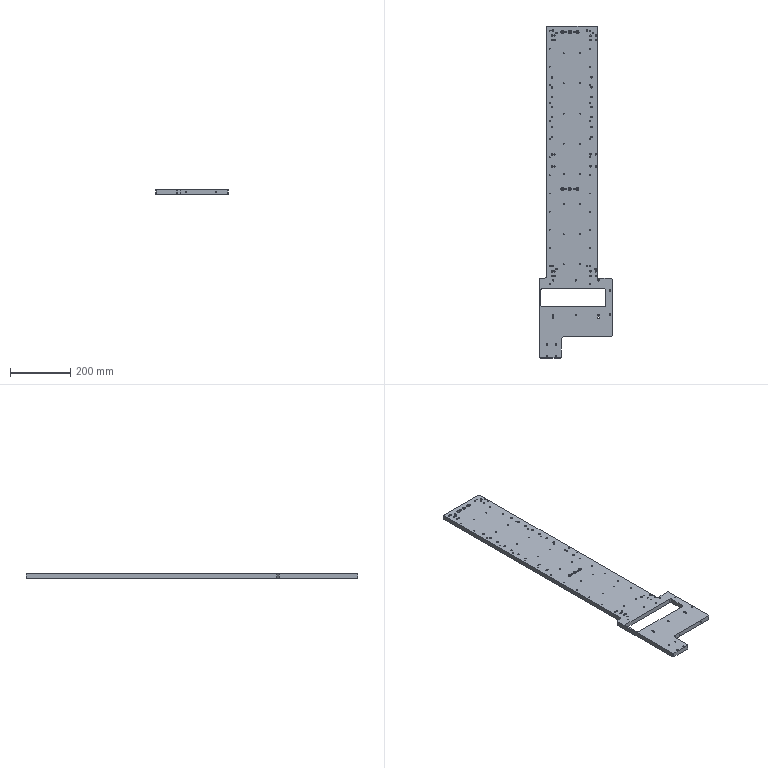Part | STEP file | 11-FG-B07211 | 1 solid | 343 faces | box 240 x 1100 x 15 mm | volume 2663856 mm3 | cylinder 256 | cone 60 | plane 27 | commonest cylinder face diameters 3.3 x96 5 x96 4.2 x24 10 x13 6 x8 5.5 x6